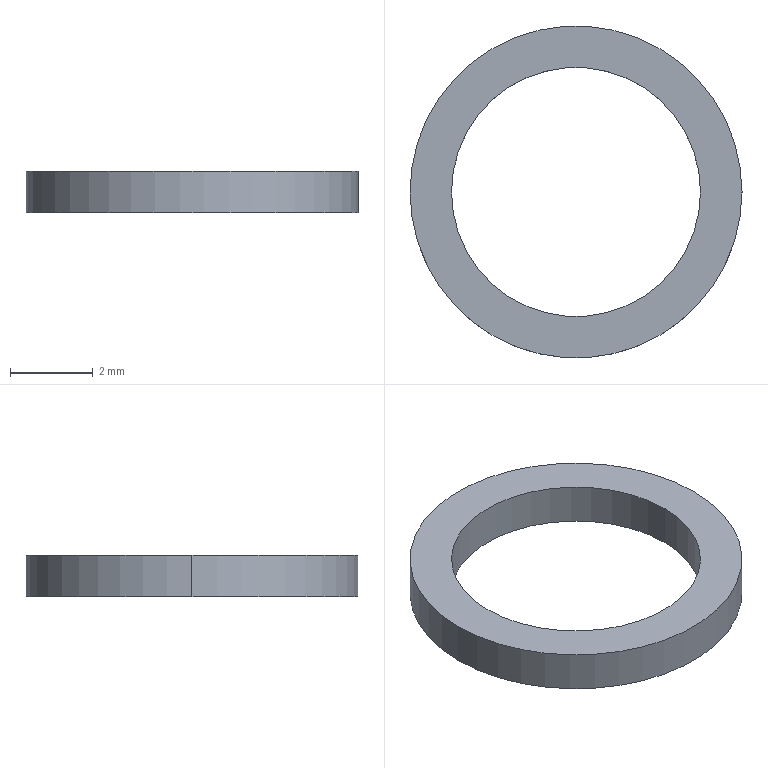Part | SolidWorks | features Extrusion 1 | 1 solid | 6 faces | box 8 x 8 x 1 mm | volume 21.991 mm3 | cylinder 4 | plane 2 | commonest cylinder face diameters 6 x2 8 x2
STEP:
#1=CARTESIAN_POINT('',(-3.,0.,1.));
#2=VERTEX_POINT('',#1);
#3=CARTESIAN_POINT('',(3.,0.,1.));
#4=VERTEX_POINT('',#3);
#5=CARTESIAN_POINT('',(0.,0.,1.));
#6=DIRECTION('',(0.,0.,1.));
#7=DIRECTION('',(1.,0.,0.));
#8=AXIS2_PLACEMENT_3D('',#5,#6,#7);
#9=CIRCLE('',#8,3.);
#10=EDGE_CURVE('',#2,#4,#9,.T.);
#11=ORIENTED_EDGE('',*,*,#10,.T.);
#12=CARTESIAN_POINT('',(3.,0.,0.));
#13=VERTEX_POINT('',#12);
#14=CARTESIAN_POINT('',(3.,0.,1.));
#15=DIRECTION('',(0.,0.,-1.));
#16=VECTOR('',#15,1000.);
#17=LINE('',#14,#16);
#18=EDGE_CURVE('',#4,#13,#17,.T.);
#19=ORIENTED_EDGE('',*,*,#18,.T.);
#20=CARTESIAN_POINT('',(-3.,0.,0.));
#21=VERTEX_POINT('',#20);
#22=CARTESIAN_POINT('',(0.,0.,0.));
#23=DIRECTION('',(0.,0.,1.));
#24=DIRECTION('',(1.,0.,0.));
#25=AXIS2_PLACEMENT_3D('',#22,#23,#24);
#26=CIRCLE('',#25,3.);
#27=EDGE_CURVE('',#21,#13,#26,.T.);
#28=ORIENTED_EDGE('',*,*,#27,.F.);
#29=CARTESIAN_POINT('',(-3.,0.,1.));
#30=DIRECTION('',(0.,0.,-1.));
#31=VECTOR('',#30,1000.);
#32=LINE('',#29,#31);
#33=EDGE_CURVE('',#2,#21,#32,.T.);
#34=ORIENTED_EDGE('',*,*,#33,.F.);
#35=EDGE_LOOP('',(#11,#19,#28,#34));
#36=FACE_OUTER_BOUND('',#35,.T.);
#37=CARTESIAN_POINT('',(0.,0.,1.));
#38=DIRECTION('',(0.,0.,-1.));
#39=DIRECTION('',(-1.,0.,0.));
#40=AXIS2_PLACEMENT_3D('',#37,#38,#39);
#41=CYLINDRICAL_SURFACE('',#40,3.);
#42=ADVANCED_FACE('',(#36),#41,.F.);
#43=CARTESIAN_POINT('',(4.,0.,1.));
#44=VERTEX_POINT('',#43);
#45=CARTESIAN_POINT('',(-4.,0.,1.));
#46=VERTEX_POINT('',#45);
#47=CARTESIAN_POINT('',(0.,0.,1.));
#48=DIRECTION('',(0.,0.,1.));
#49=DIRECTION('',(1.,0.,0.));
#50=AXIS2_PLACEMENT_3D('',#47,#48,#49);
#51=CIRCLE('',#50,4.);
#52=EDGE_CURVE('',#44,#46,#51,.T.);
#53=ORIENTED_EDGE('',*,*,#52,.F.);
#54=CARTESIAN_POINT('',(4.,0.,0.));
#55=VERTEX_POINT('',#54);
#56=CARTESIAN_POINT('',(4.,0.,1.));
#57=DIRECTION('',(0.,0.,-1.));
#58=VECTOR('',#57,1000.);
#59=LINE('',#56,#58);
#60=EDGE_CURVE('',#44,#55,#59,.T.);
#61=ORIENTED_EDGE('',*,*,#60,.T.);
#62=CARTESIAN_POINT('',(-4.,0.,0.));
#63=VERTEX_POINT('',#62);
#64=CARTESIAN_POINT('',(0.,0.,0.));
#65=DIRECTION('',(0.,0.,1.));
#66=DIRECTION('',(1.,0.,0.));
#67=AXIS2_PLACEMENT_3D('',#64,#65,#66);
#68=CIRCLE('',#67,4.);
#69=EDGE_CURVE('',#55,#63,#68,.T.);
#70=ORIENTED_EDGE('',*,*,#69,.T.);
#71=CARTESIAN_POINT('',(-4.,0.,1.));
#72=DIRECTION('',(0.,0.,-1.));
#73=VECTOR('',#72,1000.);
#74=LINE('',#71,#73);
#75=EDGE_CURVE('',#46,#63,#74,.T.);
#76=ORIENTED_EDGE('',*,*,#75,.F.);
#77=EDGE_LOOP('',(#53,#61,#70,#76));
#78=FACE_OUTER_BOUND('',#77,.T.);
#79=CARTESIAN_POINT('',(0.,0.,1.));
#80=DIRECTION('',(0.,0.,-1.));
#81=DIRECTION('',(-1.,0.,0.));
#82=AXIS2_PLACEMENT_3D('',#79,#80,#81);
#83=CYLINDRICAL_SURFACE('',#82,4.);
#84=ADVANCED_FACE('',(#78),#83,.T.);
#85=CARTESIAN_POINT('',(0.,0.,1.));
#86=DIRECTION('',(0.,0.,1.));
#87=DIRECTION('',(1.,0.,0.));
#88=AXIS2_PLACEMENT_3D('',#85,#86,#87);
#89=CIRCLE('',#88,4.);
#90=EDGE_CURVE('',#46,#44,#89,.T.);
#91=ORIENTED_EDGE('',*,*,#90,.T.);
#92=ORIENTED_EDGE('',*,*,#52,.T.);
#93=EDGE_LOOP('',(#91,#92));
#94=FACE_OUTER_BOUND('',#93,.T.);
#95=ORIENTED_EDGE('',*,*,#10,.F.);
#96=CARTESIAN_POINT('',(0.,0.,1.));
#97=DIRECTION('',(0.,0.,1.));
#98=DIRECTION('',(1.,0.,0.));
#99=AXIS2_PLACEMENT_3D('',#96,#97,#98);
#100=CIRCLE('',#99,3.);
#101=EDGE_CURVE('',#4,#2,#100,.T.);
#102=ORIENTED_EDGE('',*,*,#101,.F.);
#103=EDGE_LOOP('',(#95,#102));
#104=FACE_BOUND('',#103,.T.);
#105=CARTESIAN_POINT('',(0.,0.,1.));
#106=DIRECTION('',(0.,0.,1.));
#107=DIRECTION('',(1.,0.,0.));
#108=AXIS2_PLACEMENT_3D('',#105,#106,#107);
#109=PLANE('',#108);
#110=ADVANCED_FACE('',(#94,#104),#109,.T.);
#111=CARTESIAN_POINT('',(0.,0.,0.));
#112=DIRECTION('',(0.,0.,1.));
#113=DIRECTION('',(1.,0.,0.));
#114=AXIS2_PLACEMENT_3D('',#111,#112,#113);
#115=CIRCLE('',#114,4.);
#116=EDGE_CURVE('',#63,#55,#115,.T.);
#117=ORIENTED_EDGE('',*,*,#116,.F.);
#118=ORIENTED_EDGE('',*,*,#69,.F.);
#119=EDGE_LOOP('',(#117,#118));
#120=FACE_OUTER_BOUND('',#119,.T.);
#121=ORIENTED_EDGE('',*,*,#27,.T.);
#122=CARTESIAN_POINT('',(0.,0.,0.));
#123=DIRECTION('',(0.,0.,1.));
#124=DIRECTION('',(1.,0.,0.));
#125=AXIS2_PLACEMENT_3D('',#122,#123,#124);
#126=CIRCLE('',#125,3.);
#127=EDGE_CURVE('',#13,#21,#126,.T.);
#128=ORIENTED_EDGE('',*,*,#127,.T.);
#129=EDGE_LOOP('',(#121,#128));
#130=FACE_BOUND('',#129,.T.);
#131=CARTESIAN_POINT('',(0.,0.,0.));
#132=DIRECTION('',(0.,0.,1.));
#133=DIRECTION('',(1.,0.,0.));
#134=AXIS2_PLACEMENT_3D('',#131,#132,#133);
#135=PLANE('',#134);
#136=ADVANCED_FACE('',(#120,#130),#135,.F.);
#137=ORIENTED_EDGE('',*,*,#60,.F.);
#138=ORIENTED_EDGE('',*,*,#90,.F.);
#139=ORIENTED_EDGE('',*,*,#75,.T.);
#140=ORIENTED_EDGE('',*,*,#116,.T.);
#141=EDGE_LOOP('',(#137,#138,#139,#140));
#142=FACE_OUTER_BOUND('',#141,.T.);
#143=CARTESIAN_POINT('',(0.,0.,1.));
#144=DIRECTION('',(0.,0.,-1.));
#145=DIRECTION('',(-1.,0.,0.));
#146=AXIS2_PLACEMENT_3D('',#143,#144,#145);
#147=CYLINDRICAL_SURFACE('',#146,4.);
#148=ADVANCED_FACE('',(#142),#147,.T.);
#149=ORIENTED_EDGE('',*,*,#18,.F.);
#150=ORIENTED_EDGE('',*,*,#101,.T.);
#151=ORIENTED_EDGE('',*,*,#33,.T.);
#152=ORIENTED_EDGE('',*,*,#127,.F.);
#153=EDGE_LOOP('',(#149,#150,#151,#152));
#154=FACE_OUTER_BOUND('',#153,.T.);
#155=CARTESIAN_POINT('',(0.,0.,1.));
#156=DIRECTION('',(0.,0.,-1.));
#157=DIRECTION('',(-1.,0.,0.));
#158=AXIS2_PLACEMENT_3D('',#155,#156,#157);
#159=CYLINDRICAL_SURFACE('',#158,3.);
#160=ADVANCED_FACE('',(#154),#159,.F.);
#161=CLOSED_SHELL('',(#42,#84,#110,#136,#148,#160));
#162=MANIFOLD_SOLID_BREP('',#161);
#163=CARTESIAN_POINT('',(0.,0.,0.));
#164=DIRECTION('',(0.,0.,1.));
#165=DIRECTION('',(1.,0.,0.));
#166=AXIS2_PLACEMENT_3D('',#163,#164,#165);
#167=(LENGTH_UNIT()NAMED_UNIT(*)SI_UNIT(.MILLI.,.METRE.));
#168=UNCERTAINTY_MEASURE_WITH_UNIT(LENGTH_MEASURE(0.00001),#167,'','');
#169=(NAMED_UNIT(*)PLANE_ANGLE_UNIT()SI_UNIT($,.RADIAN.));
#170=(NAMED_UNIT(*)SI_UNIT($,.STERADIAN.)SOLID_ANGLE_UNIT());
#171=(GEOMETRIC_REPRESENTATION_CONTEXT(3)GLOBAL_UNCERTAINTY_ASSIGNED_CONTEXT((#168))GLOBAL_UNIT_ASSIGNED_CONTEXT((#167,#169,#170))REPRESENTATION_CONTEXT('',''));
#172=ADVANCED_BREP_SHAPE_REPRESENTATION('',(#162,#166),#171);